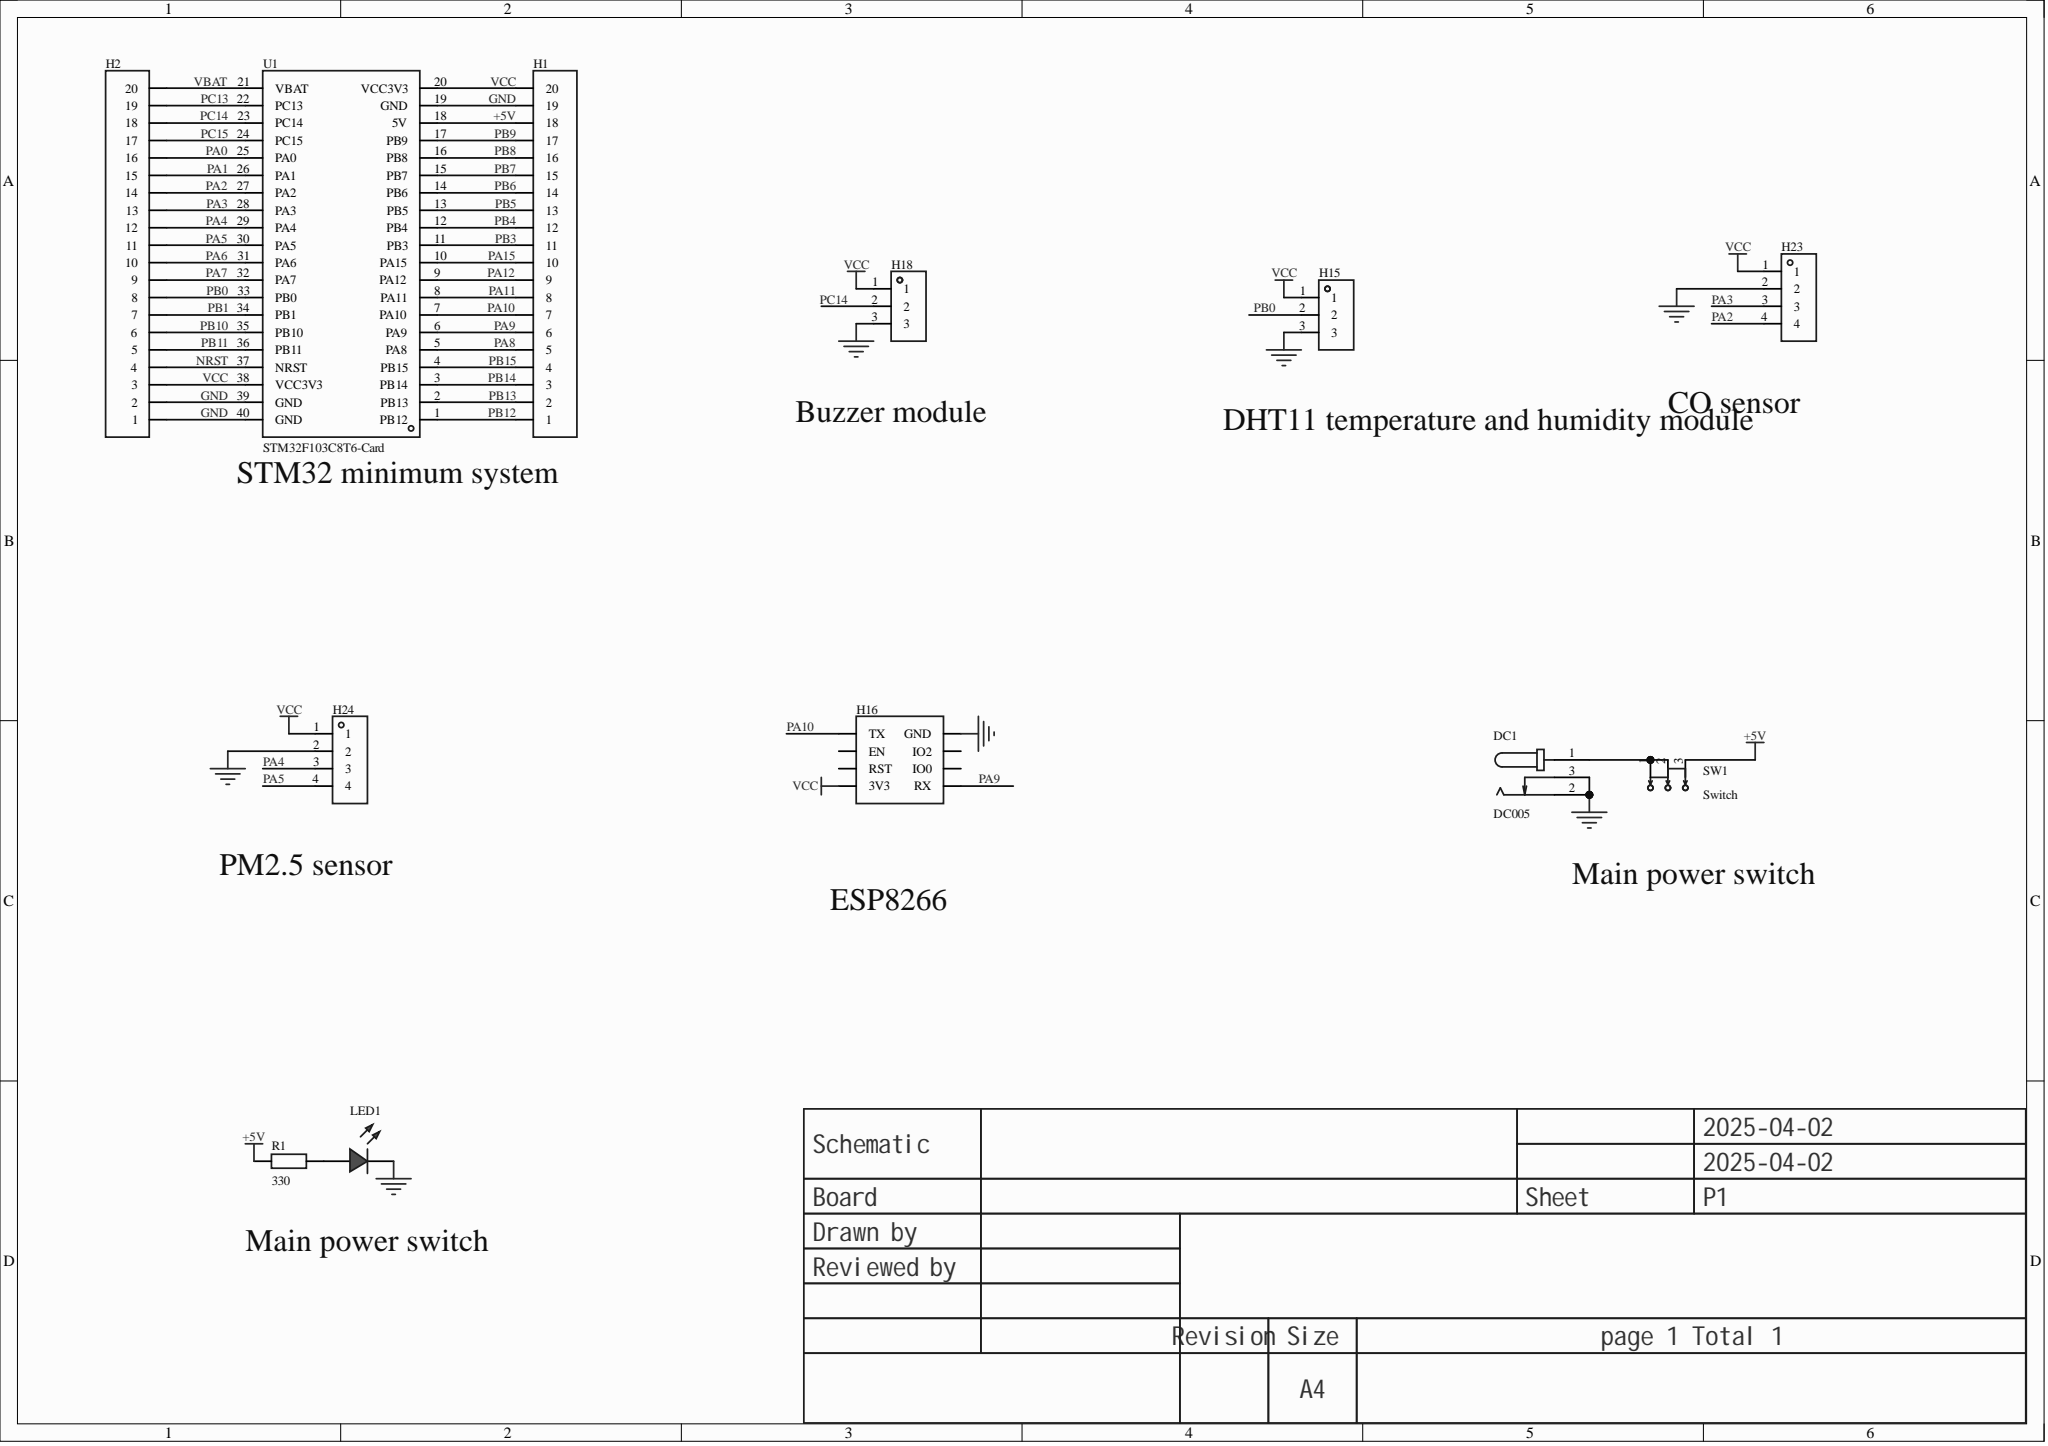Circuit board | Altium Designer | 12 parts | 39 nets
Bill of materials:
Comment,Description,Designator,Footprint,LibRef,Quantity
"DC005","Connector type: DC power socket; mounting style: right-angle; contact inner diameter: 2mm; contact outer diameter: 6.3mm; rated current: 500mA; rated voltage: 30V; operating temperature range: -25℃~+70℃;","DC1","DC-IN-TH_DC005","DC005","1"
"","","H1, H2","HDR-TH_20P-P2.54-V-F","HDR-F_2.54_1x20P","2"
"","","H15, H18","HDR-TH_3P-P2.54-V-F","HDR-F_2.54_1x3P","2"
"","","H16","HDR-TH_8P-P2.54-V-F-R2-C4-S2.54-1","HDR-F_2.54_2x4","1"
"","","H23, H24","HDR-TH_4P-P2.54-V-M","HDR-M_2.54_1x4P","2"
"","","LED1","LED_TH-3mm","LED_TH-R_3mm","1"
"330","","R1","Res_1/4W","Res_AXIAL-1/4W","1"
"Switch","","SW1","SW-TH_SS-12D01-GX","开关","1"
"STM32F103C8T6-Card","","U1","CONN-TH_L53.3-W22.9_STM32F103C8T6-CARD","STM32F103C8T6-Card","1"
Netlist (Protel format):
[
DC1
DC-IN-TH_DC005
DC005



]
[
H1
HDR-TH_20P-P2.54-V-F




]
[
H2
HDR-TH_20P-P2.54-V-F




]
[
H15
HDR-TH_3P-P2.54-V-F




]
[
H16
HDR-TH_8P-P2.54-V-F-R2-C4-S2.54-1




]
[
H18
HDR-TH_3P-P2.54-V-F




]
[
H23
HDR-TH_4P-P2.54-V-M




]
[
H24
HDR-TH_4P-P2.54-V-M




]
[
LED1
LED_TH-3mm




]
[
R1
Res_1/4W
330



]
[
SW1
SW-TH_SS-12D01-GX
Switch



]
[
U1
CONN-TH_L53.3-W22.9_STM32F103C8T6-CARD
STM32F103C8T6-Card



]
(
VCC
H1-20
H2-3
H15-1
H16-7
H18-1
H23-1
H24-1
U1-20
U1-38
)
(
VBAT
H2-20
U1-21
)
(
PC15
H2-17
U1-24
)
(
PC14
H2-18
H18-2
U1-23
)
(
PC13
H2-19
U1-22
)
(
PB15
H1-4
U1-4
)
(
PB14
H1-3
U1-3
)
(
PB13
H1-2
U1-2
)
(
PB12
H1-1
U1-1
)
(
PB11
H2-5
U1-36
)
(
PB10
H2-6
U1-35
)
(
PB9
H1-17
U1-17
)
(
PB8
H1-16
U1-16
)
(
PB7
H1-15
U1-15
)
(
PB6
H1-14
U1-14
)
(
PB5
H1-13
U1-13
)
(
PB4
H1-12
U1-12
)
(
PB3
H1-11
U1-11
)
(
PB1
H2-7
U1-34
)
(
PB0
H2-8
H15-2
U1-33
)
(
PA15
H1-10
U1-10
)
(
PA12
H1-9
U1-9
)
(
PA11
H1-8
U1-8
)
(
PA10
H1-7
H16-1
U1-7
)
(
PA9
H1-6
H16-8
U1-6
)
(
PA8
H1-5
U1-5
)
(
PA7
H2-9
U1-32
)
(
PA6
H2-10
U1-31
)
(
PA5
H2-11
H24-4
U1-30
)
(
PA4
H2-12
H24-3
U1-29
)
(
PA3
H2-13
H23-3
U1-28
)
(
PA2
H2-14
H23-4
U1-27
)
(
PA1
H2-15
U1-26
)
(
PA0
H2-16
U1-25
)
(
NRST
H2-4
U1-37
)
(
NetLED1_1
LED1-1
R1-2
)
(
NetDC1_1
DC1-1
SW1-1
SW1-2
)
(
GND
DC1-2
DC1-3
H1-19
H2-1
H2-2
H15-3
H16-2
H18-3
H23-2
H24-2
LED1-2
U1-19
U1-39
U1-40
)
(
+5V
H1-18
R1-1
SW1-3
U1-18
)